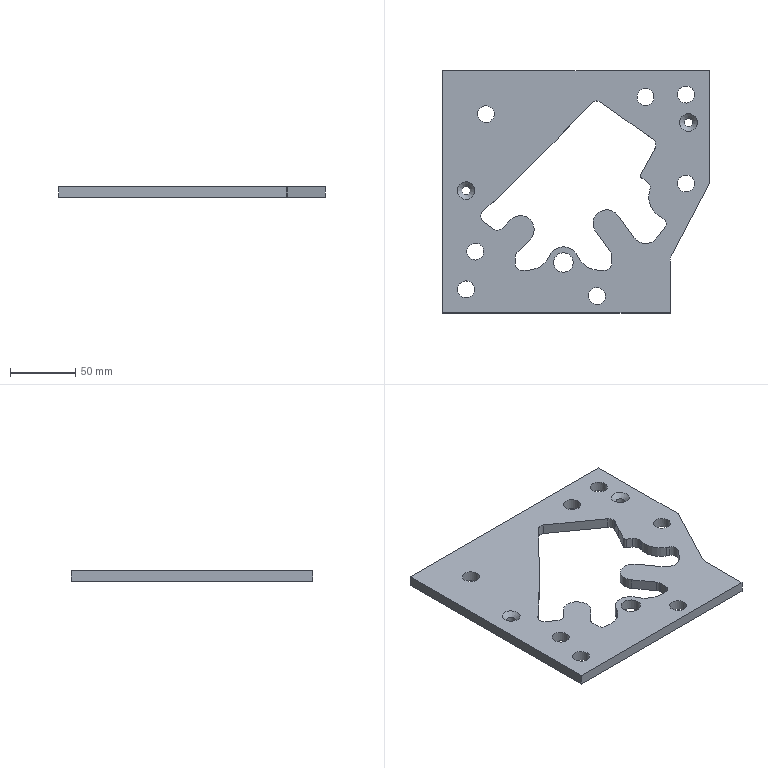Part | STEP file | gslz 2016.10.28-13_id126_x_t | 1 solid | 61 faces | box 204 x 185 x 8 mm | volume 197619 mm3 | cylinder 30 | plane 29 | cone 2 | commonest cylinder face diameters 10 x9 13 x7 6.5 x2 21 x2 36 x2 4 x1